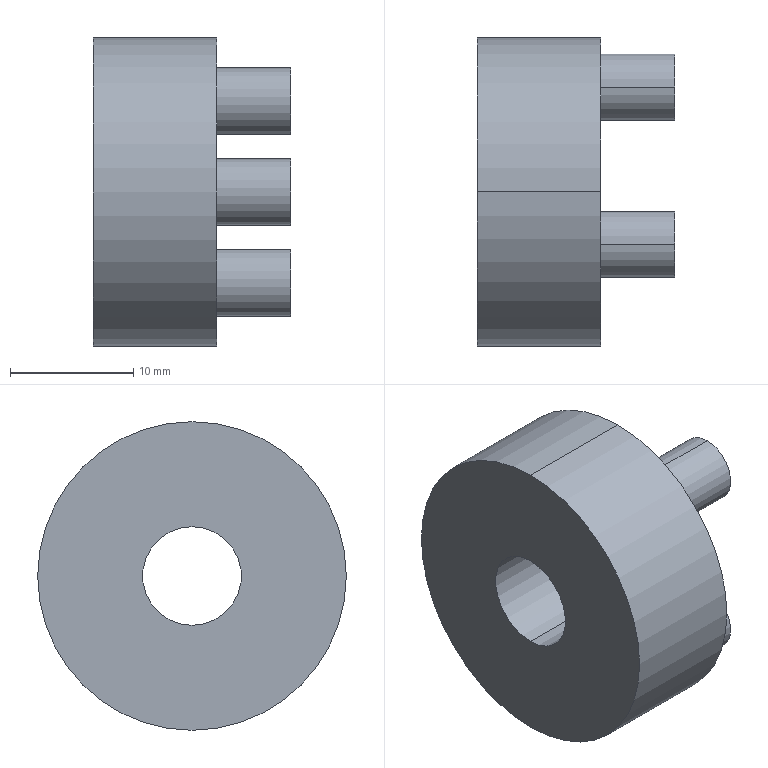Part | SolidWorks | features BaseBody 1 | 1 solid | 15 faces | box 16 x 25 x 25 mm | volume 4818 mm3 | cylinder 10 | plane 5 | commonest cylinder face diameters 5.4 x6 8 x2 25 x2
STEP:
#1=CARTESIAN_POINT('',(-5.,0.,-12.5));
#2=VERTEX_POINT('',#1);
#3=CARTESIAN_POINT('',(-5.,0.,12.5));
#4=VERTEX_POINT('',#3);
#5=CARTESIAN_POINT('',(-5.,0.,0.));
#6=DIRECTION('',(1.,0.,0.));
#7=DIRECTION('',(0.,0.,-1.));
#8=AXIS2_PLACEMENT_3D('',#5,#6,#7);
#9=CIRCLE('',#8,12.5);
#10=EDGE_CURVE('',#2,#4,#9,.T.);
#11=ORIENTED_EDGE('',*,*,#10,.T.);
#12=CARTESIAN_POINT('',(5.,0.,12.5));
#13=VERTEX_POINT('',#12);
#14=CARTESIAN_POINT('',(-5.,0.,12.5));
#15=DIRECTION('',(1.,0.,0.));
#16=VECTOR('',#15,1000.);
#17=LINE('',#14,#16);
#18=EDGE_CURVE('',#4,#13,#17,.T.);
#19=ORIENTED_EDGE('',*,*,#18,.T.);
#20=CARTESIAN_POINT('',(5.,0.,-12.5));
#21=VERTEX_POINT('',#20);
#22=CARTESIAN_POINT('',(5.,0.,0.));
#23=DIRECTION('',(-1.,0.,0.));
#24=DIRECTION('',(0.,0.,-1.));
#25=AXIS2_PLACEMENT_3D('',#22,#23,#24);
#26=CIRCLE('',#25,12.5);
#27=EDGE_CURVE('',#13,#21,#26,.T.);
#28=ORIENTED_EDGE('',*,*,#27,.T.);
#29=CARTESIAN_POINT('',(-5.,0.,-12.5));
#30=DIRECTION('',(1.,0.,0.));
#31=VECTOR('',#30,1000.);
#32=LINE('',#29,#31);
#33=EDGE_CURVE('',#2,#21,#32,.T.);
#34=ORIENTED_EDGE('',*,*,#33,.F.);
#35=EDGE_LOOP('',(#11,#19,#28,#34));
#36=FACE_OUTER_BOUND('',#35,.T.);
#37=CARTESIAN_POINT('',(-5.,0.,0.));
#38=DIRECTION('',(1.,0.,0.));
#39=DIRECTION('',(0.,0.,-1.));
#40=AXIS2_PLACEMENT_3D('',#37,#38,#39);
#41=CYLINDRICAL_SURFACE('',#40,12.5);
#42=ADVANCED_FACE('',(#36),#41,.T.);
#43=CARTESIAN_POINT('',(-5.,0.,-4.));
#44=VERTEX_POINT('',#43);
#45=CARTESIAN_POINT('',(-5.,0.,4.));
#46=VERTEX_POINT('',#45);
#47=CARTESIAN_POINT('',(-5.,0.,0.));
#48=DIRECTION('',(-1.,0.,0.));
#49=DIRECTION('',(0.,0.,-1.));
#50=AXIS2_PLACEMENT_3D('',#47,#48,#49);
#51=CIRCLE('',#50,4.);
#52=EDGE_CURVE('',#44,#46,#51,.T.);
#53=ORIENTED_EDGE('',*,*,#52,.T.);
#54=CARTESIAN_POINT('',(5.,0.,4.));
#55=VERTEX_POINT('',#54);
#56=CARTESIAN_POINT('',(-6.,0.,4.));
#57=DIRECTION('',(1.,0.,0.));
#58=VECTOR('',#57,1000.);
#59=LINE('',#56,#58);
#60=EDGE_CURVE('',#46,#55,#59,.T.);
#61=ORIENTED_EDGE('',*,*,#60,.T.);
#62=CARTESIAN_POINT('',(5.,0.,-4.));
#63=VERTEX_POINT('',#62);
#64=CARTESIAN_POINT('',(5.,0.,0.));
#65=DIRECTION('',(-1.,0.,0.));
#66=DIRECTION('',(0.,0.,-1.));
#67=AXIS2_PLACEMENT_3D('',#64,#65,#66);
#68=CIRCLE('',#67,4.);
#69=EDGE_CURVE('',#63,#55,#68,.T.);
#70=ORIENTED_EDGE('',*,*,#69,.F.);
#71=CARTESIAN_POINT('',(-6.,0.,-4.));
#72=DIRECTION('',(1.,0.,0.));
#73=VECTOR('',#72,1000.);
#74=LINE('',#71,#73);
#75=EDGE_CURVE('',#44,#63,#74,.T.);
#76=ORIENTED_EDGE('',*,*,#75,.F.);
#77=EDGE_LOOP('',(#53,#61,#70,#76));
#78=FACE_OUTER_BOUND('',#77,.T.);
#79=CARTESIAN_POINT('',(-6.,0.,0.));
#80=DIRECTION('',(1.,0.,0.));
#81=DIRECTION('',(0.,0.,-1.));
#82=AXIS2_PLACEMENT_3D('',#79,#80,#81);
#83=CYLINDRICAL_SURFACE('',#82,4.);
#84=ADVANCED_FACE('',(#78),#83,.F.);
#85=CARTESIAN_POINT('',(5.,8.5,2.7));
#86=VERTEX_POINT('',#85);
#87=CARTESIAN_POINT('',(5.,8.5,-2.7));
#88=VERTEX_POINT('',#87);
#89=CARTESIAN_POINT('',(5.,8.5,0.));
#90=DIRECTION('',(-1.,0.,0.));
#91=DIRECTION('',(0.,0.,-1.));
#92=AXIS2_PLACEMENT_3D('',#89,#90,#91);
#93=CIRCLE('',#92,2.7);
#94=EDGE_CURVE('',#86,#88,#93,.T.);
#95=ORIENTED_EDGE('',*,*,#94,.F.);
#96=CARTESIAN_POINT('',(11.,8.5,2.7));
#97=VERTEX_POINT('',#96);
#98=CARTESIAN_POINT('',(5.,8.5,2.7));
#99=DIRECTION('',(1.,0.,0.));
#100=VECTOR('',#99,1000.);
#101=LINE('',#98,#100);
#102=EDGE_CURVE('',#86,#97,#101,.T.);
#103=ORIENTED_EDGE('',*,*,#102,.T.);
#104=CARTESIAN_POINT('',(11.,8.5,-2.7));
#105=VERTEX_POINT('',#104);
#106=CARTESIAN_POINT('',(11.,8.5,0.));
#107=DIRECTION('',(-1.,0.,0.));
#108=DIRECTION('',(0.,0.,-1.));
#109=AXIS2_PLACEMENT_3D('',#106,#107,#108);
#110=CIRCLE('',#109,2.7);
#111=EDGE_CURVE('',#97,#105,#110,.T.);
#112=ORIENTED_EDGE('',*,*,#111,.T.);
#113=CARTESIAN_POINT('',(5.,8.5,-2.7));
#114=DIRECTION('',(1.,0.,0.));
#115=VECTOR('',#114,1000.);
#116=LINE('',#113,#115);
#117=EDGE_CURVE('',#88,#105,#116,.T.);
#118=ORIENTED_EDGE('',*,*,#117,.F.);
#119=EDGE_LOOP('',(#95,#103,#112,#118));
#120=FACE_OUTER_BOUND('',#119,.T.);
#121=CARTESIAN_POINT('',(5.,8.5,0.));
#122=DIRECTION('',(1.,0.,0.));
#123=DIRECTION('',(0.,0.,-1.));
#124=AXIS2_PLACEMENT_3D('',#121,#122,#123);
#125=CYLINDRICAL_SURFACE('',#124,2.7);
#126=ADVANCED_FACE('',(#120),#125,.T.);
#127=CARTESIAN_POINT('',(5.,-4.25,-4.661));
#128=VERTEX_POINT('',#127);
#129=CARTESIAN_POINT('',(5.,-4.25,-10.061));
#130=VERTEX_POINT('',#129);
#131=CARTESIAN_POINT('',(5.,-4.25,-7.361));
#132=DIRECTION('',(-1.,0.,0.));
#133=DIRECTION('',(0.,0.,-1.));
#134=AXIS2_PLACEMENT_3D('',#131,#132,#133);
#135=CIRCLE('',#134,2.7);
#136=EDGE_CURVE('',#128,#130,#135,.T.);
#137=ORIENTED_EDGE('',*,*,#136,.F.);
#138=CARTESIAN_POINT('',(11.,-4.25,-4.661));
#139=VERTEX_POINT('',#138);
#140=CARTESIAN_POINT('',(5.,-4.25,-4.661));
#141=DIRECTION('',(1.,0.,0.));
#142=VECTOR('',#141,1000.);
#143=LINE('',#140,#142);
#144=EDGE_CURVE('',#128,#139,#143,.T.);
#145=ORIENTED_EDGE('',*,*,#144,.T.);
#146=CARTESIAN_POINT('',(11.,-4.25,-10.061));
#147=VERTEX_POINT('',#146);
#148=CARTESIAN_POINT('',(11.,-4.25,-7.361));
#149=DIRECTION('',(-1.,0.,0.));
#150=DIRECTION('',(0.,0.,-1.));
#151=AXIS2_PLACEMENT_3D('',#148,#149,#150);
#152=CIRCLE('',#151,2.7);
#153=EDGE_CURVE('',#139,#147,#152,.T.);
#154=ORIENTED_EDGE('',*,*,#153,.T.);
#155=CARTESIAN_POINT('',(5.,-4.25,-10.061));
#156=DIRECTION('',(1.,0.,0.));
#157=VECTOR('',#156,1000.);
#158=LINE('',#155,#157);
#159=EDGE_CURVE('',#130,#147,#158,.T.);
#160=ORIENTED_EDGE('',*,*,#159,.F.);
#161=EDGE_LOOP('',(#137,#145,#154,#160));
#162=FACE_OUTER_BOUND('',#161,.T.);
#163=CARTESIAN_POINT('',(5.,-4.25,-7.361));
#164=DIRECTION('',(1.,0.,0.));
#165=DIRECTION('',(0.,0.,-1.));
#166=AXIS2_PLACEMENT_3D('',#163,#164,#165);
#167=CYLINDRICAL_SURFACE('',#166,2.7);
#168=ADVANCED_FACE('',(#162),#167,.T.);
#169=CARTESIAN_POINT('',(5.,-4.25,10.061));
#170=VERTEX_POINT('',#169);
#171=CARTESIAN_POINT('',(5.,-4.25,4.661));
#172=VERTEX_POINT('',#171);
#173=CARTESIAN_POINT('',(5.,-4.25,7.361));
#174=DIRECTION('',(-1.,0.,0.));
#175=DIRECTION('',(0.,0.,-1.));
#176=AXIS2_PLACEMENT_3D('',#173,#174,#175);
#177=CIRCLE('',#176,2.7);
#178=EDGE_CURVE('',#170,#172,#177,.T.);
#179=ORIENTED_EDGE('',*,*,#178,.F.);
#180=CARTESIAN_POINT('',(11.,-4.25,10.061));
#181=VERTEX_POINT('',#180);
#182=CARTESIAN_POINT('',(5.,-4.25,10.061));
#183=DIRECTION('',(1.,0.,0.));
#184=VECTOR('',#183,1000.);
#185=LINE('',#182,#184);
#186=EDGE_CURVE('',#170,#181,#185,.T.);
#187=ORIENTED_EDGE('',*,*,#186,.T.);
#188=CARTESIAN_POINT('',(11.,-4.25,4.661));
#189=VERTEX_POINT('',#188);
#190=CARTESIAN_POINT('',(11.,-4.25,7.361));
#191=DIRECTION('',(-1.,0.,0.));
#192=DIRECTION('',(0.,0.,-1.));
#193=AXIS2_PLACEMENT_3D('',#190,#191,#192);
#194=CIRCLE('',#193,2.7);
#195=EDGE_CURVE('',#181,#189,#194,.T.);
#196=ORIENTED_EDGE('',*,*,#195,.T.);
#197=CARTESIAN_POINT('',(5.,-4.25,4.661));
#198=DIRECTION('',(1.,0.,0.));
#199=VECTOR('',#198,1000.);
#200=LINE('',#197,#199);
#201=EDGE_CURVE('',#172,#189,#200,.T.);
#202=ORIENTED_EDGE('',*,*,#201,.F.);
#203=EDGE_LOOP('',(#179,#187,#196,#202));
#204=FACE_OUTER_BOUND('',#203,.T.);
#205=CARTESIAN_POINT('',(5.,-4.25,7.361));
#206=DIRECTION('',(1.,0.,0.));
#207=DIRECTION('',(0.,0.,-1.));
#208=AXIS2_PLACEMENT_3D('',#205,#206,#207);
#209=CYLINDRICAL_SURFACE('',#208,2.7);
#210=ADVANCED_FACE('',(#204),#209,.T.);
#211=ORIENTED_EDGE('',*,*,#18,.F.);
#212=CARTESIAN_POINT('',(-5.,0.,0.));
#213=DIRECTION('',(1.,0.,0.));
#214=DIRECTION('',(0.,0.,-1.));
#215=AXIS2_PLACEMENT_3D('',#212,#213,#214);
#216=CIRCLE('',#215,12.5);
#217=EDGE_CURVE('',#4,#2,#216,.T.);
#218=ORIENTED_EDGE('',*,*,#217,.T.);
#219=ORIENTED_EDGE('',*,*,#33,.T.);
#220=CARTESIAN_POINT('',(5.,0.,0.));
#221=DIRECTION('',(-1.,0.,0.));
#222=DIRECTION('',(0.,0.,-1.));
#223=AXIS2_PLACEMENT_3D('',#220,#221,#222);
#224=CIRCLE('',#223,12.5);
#225=EDGE_CURVE('',#21,#13,#224,.T.);
#226=ORIENTED_EDGE('',*,*,#225,.T.);
#227=EDGE_LOOP('',(#211,#218,#219,#226));
#228=FACE_OUTER_BOUND('',#227,.T.);
#229=CARTESIAN_POINT('',(-5.,0.,0.));
#230=DIRECTION('',(1.,0.,0.));
#231=DIRECTION('',(0.,0.,-1.));
#232=AXIS2_PLACEMENT_3D('',#229,#230,#231);
#233=CYLINDRICAL_SURFACE('',#232,12.5);
#234=ADVANCED_FACE('',(#228),#233,.T.);
#235=ORIENTED_EDGE('',*,*,#52,.F.);
#236=CARTESIAN_POINT('',(-5.,0.,0.));
#237=DIRECTION('',(-1.,0.,0.));
#238=DIRECTION('',(0.,0.,-1.));
#239=AXIS2_PLACEMENT_3D('',#236,#237,#238);
#240=CIRCLE('',#239,4.);
#241=EDGE_CURVE('',#46,#44,#240,.T.);
#242=ORIENTED_EDGE('',*,*,#241,.F.);
#243=EDGE_LOOP('',(#235,#242));
#244=FACE_BOUND('',#243,.T.);
#245=ORIENTED_EDGE('',*,*,#10,.F.);
#246=ORIENTED_EDGE('',*,*,#217,.F.);
#247=EDGE_LOOP('',(#245,#246));
#248=FACE_OUTER_BOUND('',#247,.T.);
#249=CARTESIAN_POINT('',(-5.,0.,0.));
#250=DIRECTION('',(1.,0.,0.));
#251=DIRECTION('',(0.,0.,-1.));
#252=AXIS2_PLACEMENT_3D('',#249,#250,#251);
#253=PLANE('',#252);
#254=ADVANCED_FACE('',(#244,#248),#253,.F.);
#255=CARTESIAN_POINT('',(5.,8.5,0.));
#256=DIRECTION('',(-1.,0.,0.));
#257=DIRECTION('',(0.,0.,-1.));
#258=AXIS2_PLACEMENT_3D('',#255,#256,#257);
#259=CIRCLE('',#258,2.7);
#260=EDGE_CURVE('',#88,#86,#259,.T.);
#261=ORIENTED_EDGE('',*,*,#260,.T.);
#262=ORIENTED_EDGE('',*,*,#94,.T.);
#263=EDGE_LOOP('',(#261,#262));
#264=FACE_BOUND('',#263,.T.);
#265=CARTESIAN_POINT('',(5.,-4.25,-7.361));
#266=DIRECTION('',(-1.,0.,0.));
#267=DIRECTION('',(0.,0.,-1.));
#268=AXIS2_PLACEMENT_3D('',#265,#266,#267);
#269=CIRCLE('',#268,2.7);
#270=EDGE_CURVE('',#130,#128,#269,.T.);
#271=ORIENTED_EDGE('',*,*,#270,.T.);
#272=ORIENTED_EDGE('',*,*,#136,.T.);
#273=EDGE_LOOP('',(#271,#272));
#274=FACE_BOUND('',#273,.T.);
#275=ORIENTED_EDGE('',*,*,#69,.T.);
#276=CARTESIAN_POINT('',(5.,0.,0.));
#277=DIRECTION('',(-1.,0.,0.));
#278=DIRECTION('',(0.,0.,-1.));
#279=AXIS2_PLACEMENT_3D('',#276,#277,#278);
#280=CIRCLE('',#279,4.);
#281=EDGE_CURVE('',#55,#63,#280,.T.);
#282=ORIENTED_EDGE('',*,*,#281,.T.);
#283=EDGE_LOOP('',(#275,#282));
#284=FACE_BOUND('',#283,.T.);
#285=CARTESIAN_POINT('',(5.,-4.25,7.361));
#286=DIRECTION('',(-1.,0.,0.));
#287=DIRECTION('',(0.,0.,-1.));
#288=AXIS2_PLACEMENT_3D('',#285,#286,#287);
#289=CIRCLE('',#288,2.7);
#290=EDGE_CURVE('',#172,#170,#289,.T.);
#291=ORIENTED_EDGE('',*,*,#290,.T.);
#292=ORIENTED_EDGE('',*,*,#178,.T.);
#293=EDGE_LOOP('',(#291,#292));
#294=FACE_BOUND('',#293,.T.);
#295=ORIENTED_EDGE('',*,*,#225,.F.);
#296=ORIENTED_EDGE('',*,*,#27,.F.);
#297=EDGE_LOOP('',(#295,#296));
#298=FACE_OUTER_BOUND('',#297,.T.);
#299=CARTESIAN_POINT('',(5.,0.,0.));
#300=DIRECTION('',(1.,0.,0.));
#301=DIRECTION('',(0.,0.,-1.));
#302=AXIS2_PLACEMENT_3D('',#299,#300,#301);
#303=PLANE('',#302);
#304=ADVANCED_FACE('',(#264,#274,#284,#294,#298),#303,.T.);
#305=ORIENTED_EDGE('',*,*,#60,.F.);
#306=ORIENTED_EDGE('',*,*,#241,.T.);
#307=ORIENTED_EDGE('',*,*,#75,.T.);
#308=ORIENTED_EDGE('',*,*,#281,.F.);
#309=EDGE_LOOP('',(#305,#306,#307,#308));
#310=FACE_OUTER_BOUND('',#309,.T.);
#311=CARTESIAN_POINT('',(-6.,0.,0.));
#312=DIRECTION('',(1.,0.,0.));
#313=DIRECTION('',(0.,0.,-1.));
#314=AXIS2_PLACEMENT_3D('',#311,#312,#313);
#315=CYLINDRICAL_SURFACE('',#314,4.);
#316=ADVANCED_FACE('',(#310),#315,.F.);
#317=ORIENTED_EDGE('',*,*,#102,.F.);
#318=ORIENTED_EDGE('',*,*,#260,.F.);
#319=ORIENTED_EDGE('',*,*,#117,.T.);
#320=CARTESIAN_POINT('',(11.,8.5,0.));
#321=DIRECTION('',(-1.,0.,0.));
#322=DIRECTION('',(0.,0.,-1.));
#323=AXIS2_PLACEMENT_3D('',#320,#321,#322);
#324=CIRCLE('',#323,2.7);
#325=EDGE_CURVE('',#105,#97,#324,.T.);
#326=ORIENTED_EDGE('',*,*,#325,.T.);
#327=EDGE_LOOP('',(#317,#318,#319,#326));
#328=FACE_OUTER_BOUND('',#327,.T.);
#329=CARTESIAN_POINT('',(5.,8.5,0.));
#330=DIRECTION('',(1.,0.,0.));
#331=DIRECTION('',(0.,0.,-1.));
#332=AXIS2_PLACEMENT_3D('',#329,#330,#331);
#333=CYLINDRICAL_SURFACE('',#332,2.7);
#334=ADVANCED_FACE('',(#328),#333,.T.);
#335=ORIENTED_EDGE('',*,*,#144,.F.);
#336=ORIENTED_EDGE('',*,*,#270,.F.);
#337=ORIENTED_EDGE('',*,*,#159,.T.);
#338=CARTESIAN_POINT('',(11.,-4.25,-7.361));
#339=DIRECTION('',(-1.,0.,0.));
#340=DIRECTION('',(0.,0.,-1.));
#341=AXIS2_PLACEMENT_3D('',#338,#339,#340);
#342=CIRCLE('',#341,2.7);
#343=EDGE_CURVE('',#147,#139,#342,.T.);
#344=ORIENTED_EDGE('',*,*,#343,.T.);
#345=EDGE_LOOP('',(#335,#336,#337,#344));
#346=FACE_OUTER_BOUND('',#345,.T.);
#347=CARTESIAN_POINT('',(5.,-4.25,-7.361));
#348=DIRECTION('',(1.,0.,0.));
#349=DIRECTION('',(0.,0.,-1.));
#350=AXIS2_PLACEMENT_3D('',#347,#348,#349);
#351=CYLINDRICAL_SURFACE('',#350,2.7);
#352=ADVANCED_FACE('',(#346),#351,.T.);
#353=ORIENTED_EDGE('',*,*,#186,.F.);
#354=ORIENTED_EDGE('',*,*,#290,.F.);
#355=ORIENTED_EDGE('',*,*,#201,.T.);
#356=CARTESIAN_POINT('',(11.,-4.25,7.361));
#357=DIRECTION('',(-1.,0.,0.));
#358=DIRECTION('',(0.,0.,-1.));
#359=AXIS2_PLACEMENT_3D('',#356,#357,#358);
#360=CIRCLE('',#359,2.7);
#361=EDGE_CURVE('',#189,#181,#360,.T.);
#362=ORIENTED_EDGE('',*,*,#361,.T.);
#363=EDGE_LOOP('',(#353,#354,#355,#362));
#364=FACE_OUTER_BOUND('',#363,.T.);
#365=CARTESIAN_POINT('',(5.,-4.25,7.361));
#366=DIRECTION('',(1.,0.,0.));
#367=DIRECTION('',(0.,0.,-1.));
#368=AXIS2_PLACEMENT_3D('',#365,#366,#367);
#369=CYLINDRICAL_SURFACE('',#368,2.7);
#370=ADVANCED_FACE('',(#364),#369,.T.);
#371=ORIENTED_EDGE('',*,*,#325,.F.);
#372=ORIENTED_EDGE('',*,*,#111,.F.);
#373=EDGE_LOOP('',(#371,#372));
#374=FACE_OUTER_BOUND('',#373,.T.);
#375=CARTESIAN_POINT('',(11.,8.5,0.));
#376=DIRECTION('',(1.,0.,0.));
#377=DIRECTION('',(0.,0.,-1.));
#378=AXIS2_PLACEMENT_3D('',#375,#376,#377);
#379=PLANE('',#378);
#380=ADVANCED_FACE('',(#374),#379,.T.);
#381=ORIENTED_EDGE('',*,*,#343,.F.);
#382=ORIENTED_EDGE('',*,*,#153,.F.);
#383=EDGE_LOOP('',(#381,#382));
#384=FACE_OUTER_BOUND('',#383,.T.);
#385=CARTESIAN_POINT('',(11.,-4.25,-7.361));
#386=DIRECTION('',(1.,0.,0.));
#387=DIRECTION('',(0.,0.,-1.));
#388=AXIS2_PLACEMENT_3D('',#385,#386,#387);
#389=PLANE('',#388);
#390=ADVANCED_FACE('',(#384),#389,.T.);
#391=ORIENTED_EDGE('',*,*,#361,.F.);
#392=ORIENTED_EDGE('',*,*,#195,.F.);
#393=EDGE_LOOP('',(#391,#392));
#394=FACE_OUTER_BOUND('',#393,.T.);
#395=CARTESIAN_POINT('',(11.,-4.25,7.361));
#396=DIRECTION('',(1.,0.,0.));
#397=DIRECTION('',(0.,0.,-1.));
#398=AXIS2_PLACEMENT_3D('',#395,#396,#397);
#399=PLANE('',#398);
#400=ADVANCED_FACE('',(#394),#399,.T.);
#401=CLOSED_SHELL('',(#42,#84,#126,#168,#210,#234,#254,#304,#316,#334,#352,#370,#380,#390,#400));
#402=MANIFOLD_SOLID_BREP('',#401);
#403=CARTESIAN_POINT('',(0.,0.,0.));
#404=DIRECTION('',(0.,0.,1.));
#405=DIRECTION('',(1.,0.,0.));
#406=AXIS2_PLACEMENT_3D('',#403,#404,#405);
#407=(LENGTH_UNIT()NAMED_UNIT(*)SI_UNIT(.MILLI.,.METRE.));
#408=UNCERTAINTY_MEASURE_WITH_UNIT(LENGTH_MEASURE(0.00001),#407,'','');
#409=(NAMED_UNIT(*)PLANE_ANGLE_UNIT()SI_UNIT($,.RADIAN.));
#410=(NAMED_UNIT(*)SI_UNIT($,.STERADIAN.)SOLID_ANGLE_UNIT());
#411=(GEOMETRIC_REPRESENTATION_CONTEXT(3)GLOBAL_UNCERTAINTY_ASSIGNED_CONTEXT((#408))GLOBAL_UNIT_ASSIGNED_CONTEXT((#407,#409,#410))REPRESENTATION_CONTEXT('',''));
#412=ADVANCED_BREP_SHAPE_REPRESENTATION('',(#402,#406),#411);